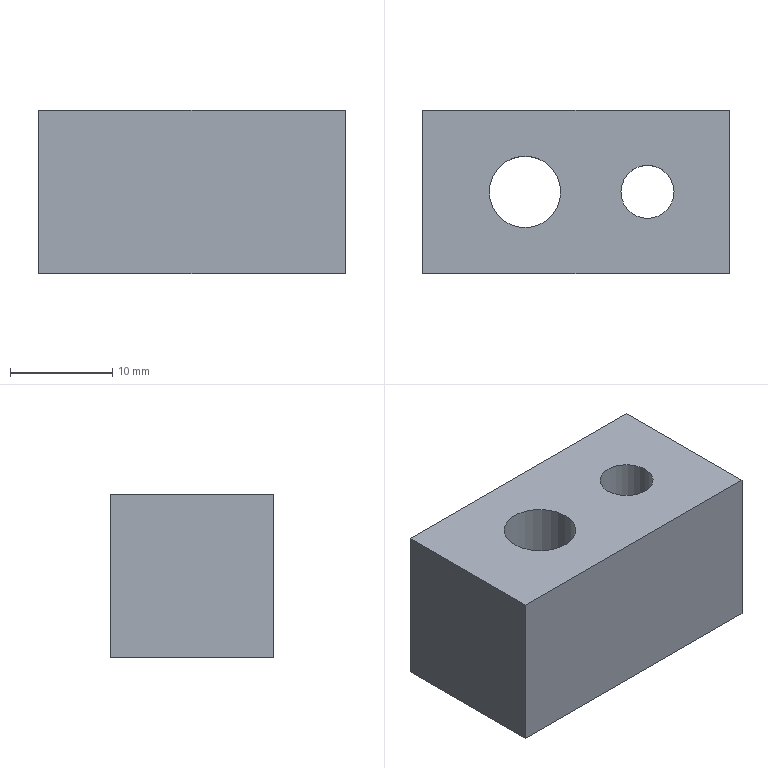Part | STEP file | PN_0012_id1934_x_t | 1 solid | 76 faces | box 30 x 16 x 16 mm | volume 6162 mm3 | plane 53 | other 19 | cylinder 4 | commonest cylinder face diameters 5.206 x1 7 x1 7.007 x1 11 x1